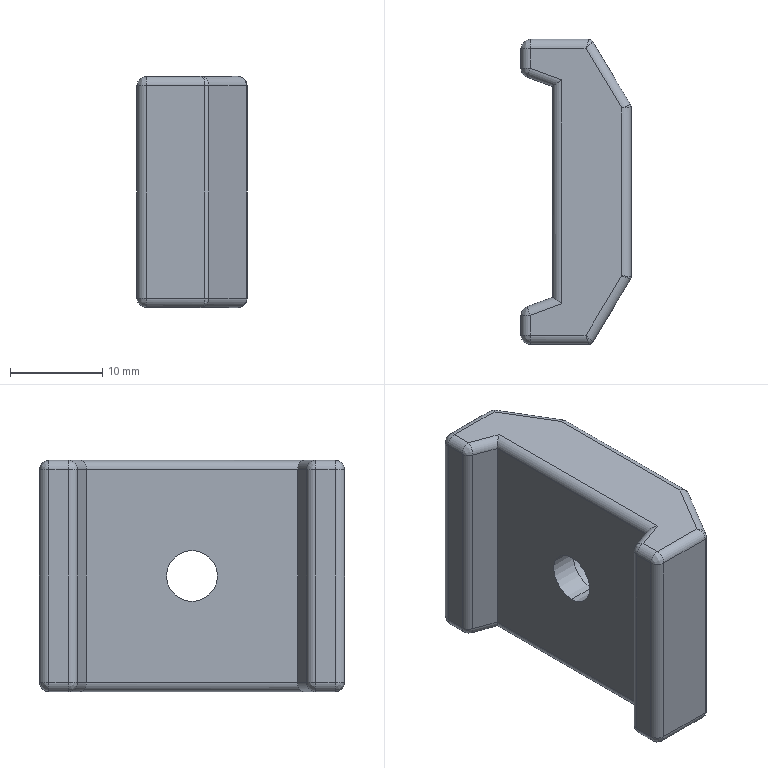Part | SolidWorks | features BaseBody 1 | 1 solid | 63 faces | box 11.9 x 33 x 25 mm | volume 6485 mm3 | cylinder 32 | spline 16 | plane 13 | cone 2 | commonest cylinder face diameters 2 x24 1 x4 5.5 x2 9.5 x2